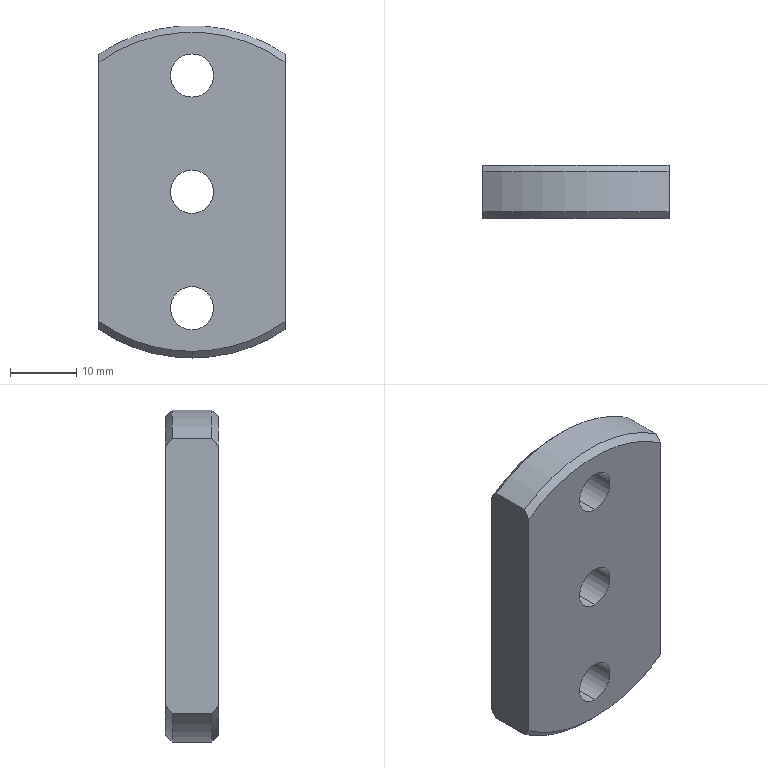Part | NX | features BREP 1 | 1 solid | 18 faces | box 28 x 8 x 50 mm | volume 9727 mm3 | cylinder 8 | cone 6 | plane 4 | commonest cylinder face diameters 6.5 x6 50 x2
STEP:
#1=CARTESIAN_POINT('',(-14.,0.,-19.494));
#2=VERTEX_POINT('',#1);
#3=CARTESIAN_POINT('',(0.,0.,-24.));
#4=VERTEX_POINT('',#3);
#5=CARTESIAN_POINT('',(0.,0.,0.));
#6=DIRECTION('',(0.,-1.,0.));
#7=DIRECTION('',(-0.5833,0.,-0.8122));
#8=AXIS2_PLACEMENT_3D('',#5,#6,#7);
#9=CIRCLE('',#8,24.);
#10=EDGE_CURVE('',#2,#4,#9,.T.);
#11=ORIENTED_EDGE('',*,*,#10,.T.);
#12=CARTESIAN_POINT('',(14.,0.,-19.494));
#13=VERTEX_POINT('',#12);
#14=CARTESIAN_POINT('',(0.,0.,0.));
#15=DIRECTION('',(0.,-1.,0.));
#16=DIRECTION('',(-0.5833,0.,-0.8122));
#17=AXIS2_PLACEMENT_3D('',#14,#15,#16);
#18=CIRCLE('',#17,24.);
#19=EDGE_CURVE('',#4,#13,#18,.T.);
#20=ORIENTED_EDGE('',*,*,#19,.T.);
#21=CARTESIAN_POINT('',(14.,0.,19.494));
#22=VERTEX_POINT('',#21);
#23=CARTESIAN_POINT('',(14.,0.,19.494));
#24=DIRECTION('',(0.,0.,-1.));
#25=VECTOR('',#24,1000.);
#26=LINE('',#23,#25);
#27=EDGE_CURVE('',#22,#13,#26,.T.);
#28=ORIENTED_EDGE('',*,*,#27,.F.);
#29=CARTESIAN_POINT('',(-14.,0.,19.494));
#30=VERTEX_POINT('',#29);
#31=CARTESIAN_POINT('',(0.,0.,0.));
#32=DIRECTION('',(0.,-1.,0.));
#33=DIRECTION('',(0.5833,0.,0.8122));
#34=AXIS2_PLACEMENT_3D('',#31,#32,#33);
#35=CIRCLE('',#34,24.);
#36=EDGE_CURVE('',#22,#30,#35,.T.);
#37=ORIENTED_EDGE('',*,*,#36,.T.);
#38=CARTESIAN_POINT('',(-14.,0.,19.494));
#39=DIRECTION('',(0.,0.,-1.));
#40=VECTOR('',#39,1000.);
#41=LINE('',#38,#40);
#42=EDGE_CURVE('',#30,#2,#41,.T.);
#43=ORIENTED_EDGE('',*,*,#42,.T.);
#44=EDGE_LOOP('',(#11,#20,#28,#37,#43));
#45=FACE_BOUND('',#44,.T.);
#46=CARTESIAN_POINT('',(0.,0.,-20.75));
#47=VERTEX_POINT('',#46);
#48=CARTESIAN_POINT('',(0.,0.,-14.25));
#49=VERTEX_POINT('',#48);
#50=CARTESIAN_POINT('',(0.,0.,-17.5));
#51=DIRECTION('',(0.,-1.,0.));
#52=DIRECTION('',(0.,0.,-1.));
#53=AXIS2_PLACEMENT_3D('',#50,#51,#52);
#54=CIRCLE('',#53,3.25);
#55=EDGE_CURVE('',#47,#49,#54,.T.);
#56=ORIENTED_EDGE('',*,*,#55,.F.);
#57=CARTESIAN_POINT('',(0.,0.,-17.5));
#58=DIRECTION('',(0.,-1.,0.));
#59=DIRECTION('',(0.,0.,1.));
#60=AXIS2_PLACEMENT_3D('',#57,#58,#59);
#61=CIRCLE('',#60,3.25);
#62=EDGE_CURVE('',#49,#47,#61,.T.);
#63=ORIENTED_EDGE('',*,*,#62,.F.);
#64=EDGE_LOOP('',(#56,#63));
#65=FACE_BOUND('',#64,.T.);
#66=CARTESIAN_POINT('',(0.,0.,20.75));
#67=VERTEX_POINT('',#66);
#68=CARTESIAN_POINT('',(0.,0.,14.25));
#69=VERTEX_POINT('',#68);
#70=CARTESIAN_POINT('',(0.,0.,17.5));
#71=DIRECTION('',(0.,-1.,0.));
#72=DIRECTION('',(0.,0.,1.));
#73=AXIS2_PLACEMENT_3D('',#70,#71,#72);
#74=CIRCLE('',#73,3.25);
#75=EDGE_CURVE('',#67,#69,#74,.T.);
#76=ORIENTED_EDGE('',*,*,#75,.F.);
#77=CARTESIAN_POINT('',(0.,0.,17.5));
#78=DIRECTION('',(0.,-1.,0.));
#79=DIRECTION('',(0.,0.,-1.));
#80=AXIS2_PLACEMENT_3D('',#77,#78,#79);
#81=CIRCLE('',#80,3.25);
#82=EDGE_CURVE('',#69,#67,#81,.T.);
#83=ORIENTED_EDGE('',*,*,#82,.F.);
#84=EDGE_LOOP('',(#76,#83));
#85=FACE_BOUND('',#84,.T.);
#86=CARTESIAN_POINT('',(0.,0.,3.25));
#87=VERTEX_POINT('',#86);
#88=CARTESIAN_POINT('',(0.,0.,-3.25));
#89=VERTEX_POINT('',#88);
#90=CARTESIAN_POINT('',(0.,0.,0.));
#91=DIRECTION('',(0.,-1.,0.));
#92=DIRECTION('',(0.,0.,1.));
#93=AXIS2_PLACEMENT_3D('',#90,#91,#92);
#94=CIRCLE('',#93,3.25);
#95=EDGE_CURVE('',#87,#89,#94,.T.);
#96=ORIENTED_EDGE('',*,*,#95,.F.);
#97=CARTESIAN_POINT('',(0.,0.,0.));
#98=DIRECTION('',(0.,-1.,0.));
#99=DIRECTION('',(0.,0.,-1.));
#100=AXIS2_PLACEMENT_3D('',#97,#98,#99);
#101=CIRCLE('',#100,3.25);
#102=EDGE_CURVE('',#89,#87,#101,.T.);
#103=ORIENTED_EDGE('',*,*,#102,.F.);
#104=EDGE_LOOP('',(#96,#103));
#105=FACE_BOUND('',#104,.T.);
#106=CARTESIAN_POINT('',(0.,0.,0.));
#107=DIRECTION('',(0.,1.,0.));
#108=DIRECTION('',(1.,0.,0.));
#109=AXIS2_PLACEMENT_3D('',#106,#107,#108);
#110=PLANE('',#109);
#111=ADVANCED_FACE('',(#45,#65,#85,#105),#110,.F.);
#112=CARTESIAN_POINT('',(0.,8.,3.25));
#113=VERTEX_POINT('',#112);
#114=CARTESIAN_POINT('',(0.,8.,3.25));
#115=DIRECTION('',(0.,-1.,0.));
#116=VECTOR('',#115,1000.);
#117=LINE('',#114,#116);
#118=EDGE_CURVE('',#87,#113,#117,.F.);
#119=ORIENTED_EDGE('',*,*,#118,.T.);
#120=CARTESIAN_POINT('',(0.,8.,-3.25));
#121=VERTEX_POINT('',#120);
#122=CARTESIAN_POINT('',(0.,8.,0.));
#123=DIRECTION('',(0.,-1.,0.));
#124=DIRECTION('',(0.,0.,-1.));
#125=AXIS2_PLACEMENT_3D('',#122,#123,#124);
#126=CIRCLE('',#125,3.25);
#127=EDGE_CURVE('',#121,#113,#126,.T.);
#128=ORIENTED_EDGE('',*,*,#127,.F.);
#129=CARTESIAN_POINT('',(0.,8.,-3.25));
#130=DIRECTION('',(0.,-1.,0.));
#131=VECTOR('',#130,1000.);
#132=LINE('',#129,#131);
#133=EDGE_CURVE('',#89,#121,#132,.F.);
#134=ORIENTED_EDGE('',*,*,#133,.F.);
#135=ORIENTED_EDGE('',*,*,#102,.T.);
#136=EDGE_LOOP('',(#119,#128,#134,#135));
#137=FACE_BOUND('',#136,.T.);
#138=CARTESIAN_POINT('',(0.,8.,0.));
#139=DIRECTION('',(0.,-1.,0.));
#140=DIRECTION('',(0.,0.,-1.));
#141=AXIS2_PLACEMENT_3D('',#138,#139,#140);
#142=CYLINDRICAL_SURFACE('',#141,3.25);
#143=ADVANCED_FACE('',(#137),#142,.F.);
#144=ORIENTED_EDGE('',*,*,#133,.T.);
#145=CARTESIAN_POINT('',(0.,8.,0.));
#146=DIRECTION('',(0.,-1.,0.));
#147=DIRECTION('',(0.,0.,1.));
#148=AXIS2_PLACEMENT_3D('',#145,#146,#147);
#149=CIRCLE('',#148,3.25);
#150=EDGE_CURVE('',#113,#121,#149,.T.);
#151=ORIENTED_EDGE('',*,*,#150,.F.);
#152=ORIENTED_EDGE('',*,*,#118,.F.);
#153=ORIENTED_EDGE('',*,*,#95,.T.);
#154=EDGE_LOOP('',(#144,#151,#152,#153));
#155=FACE_BOUND('',#154,.T.);
#156=CARTESIAN_POINT('',(0.,8.,0.));
#157=DIRECTION('',(0.,-1.,0.));
#158=DIRECTION('',(0.,0.,-1.));
#159=AXIS2_PLACEMENT_3D('',#156,#157,#158);
#160=CYLINDRICAL_SURFACE('',#159,3.25);
#161=ADVANCED_FACE('',(#155),#160,.F.);
#162=CARTESIAN_POINT('',(-14.,8.,19.494));
#163=VERTEX_POINT('',#162);
#164=CARTESIAN_POINT('',(14.,8.,19.494));
#165=VERTEX_POINT('',#164);
#166=CARTESIAN_POINT('',(0.,8.,0.));
#167=DIRECTION('',(0.,1.,0.));
#168=DIRECTION('',(-0.5833,0.,0.8122));
#169=AXIS2_PLACEMENT_3D('',#166,#167,#168);
#170=CIRCLE('',#169,24.);
#171=EDGE_CURVE('',#163,#165,#170,.T.);
#172=ORIENTED_EDGE('',*,*,#171,.T.);
#173=CARTESIAN_POINT('',(14.,8.,-19.494));
#174=VERTEX_POINT('',#173);
#175=CARTESIAN_POINT('',(14.,8.,19.494));
#176=DIRECTION('',(0.,0.,-1.));
#177=VECTOR('',#176,1000.);
#178=LINE('',#175,#177);
#179=EDGE_CURVE('',#165,#174,#178,.T.);
#180=ORIENTED_EDGE('',*,*,#179,.T.);
#181=CARTESIAN_POINT('',(0.,8.,-24.));
#182=VERTEX_POINT('',#181);
#183=CARTESIAN_POINT('',(0.,8.,0.));
#184=DIRECTION('',(0.,1.,0.));
#185=DIRECTION('',(0.5833,0.,-0.8122));
#186=AXIS2_PLACEMENT_3D('',#183,#184,#185);
#187=CIRCLE('',#186,24.);
#188=EDGE_CURVE('',#174,#182,#187,.T.);
#189=ORIENTED_EDGE('',*,*,#188,.T.);
#190=CARTESIAN_POINT('',(-14.,8.,-19.494));
#191=VERTEX_POINT('',#190);
#192=CARTESIAN_POINT('',(0.,8.,0.));
#193=DIRECTION('',(0.,1.,0.));
#194=DIRECTION('',(0.5833,0.,-0.8122));
#195=AXIS2_PLACEMENT_3D('',#192,#193,#194);
#196=CIRCLE('',#195,24.);
#197=EDGE_CURVE('',#182,#191,#196,.T.);
#198=ORIENTED_EDGE('',*,*,#197,.T.);
#199=CARTESIAN_POINT('',(-14.,8.,19.494));
#200=DIRECTION('',(0.,0.,-1.));
#201=VECTOR('',#200,1000.);
#202=LINE('',#199,#201);
#203=EDGE_CURVE('',#163,#191,#202,.T.);
#204=ORIENTED_EDGE('',*,*,#203,.F.);
#205=EDGE_LOOP('',(#172,#180,#189,#198,#204));
#206=FACE_BOUND('',#205,.T.);
#207=CARTESIAN_POINT('',(0.,8.,-20.75));
#208=VERTEX_POINT('',#207);
#209=CARTESIAN_POINT('',(0.,8.,-14.25));
#210=VERTEX_POINT('',#209);
#211=CARTESIAN_POINT('',(0.,8.,-17.5));
#212=DIRECTION('',(0.,-1.,0.));
#213=DIRECTION('',(0.,0.,-1.));
#214=AXIS2_PLACEMENT_3D('',#211,#212,#213);
#215=CIRCLE('',#214,3.25);
#216=EDGE_CURVE('',#208,#210,#215,.T.);
#217=ORIENTED_EDGE('',*,*,#216,.T.);
#218=CARTESIAN_POINT('',(0.,8.,-17.5));
#219=DIRECTION('',(0.,-1.,0.));
#220=DIRECTION('',(0.,0.,1.));
#221=AXIS2_PLACEMENT_3D('',#218,#219,#220);
#222=CIRCLE('',#221,3.25);
#223=EDGE_CURVE('',#210,#208,#222,.T.);
#224=ORIENTED_EDGE('',*,*,#223,.T.);
#225=EDGE_LOOP('',(#217,#224));
#226=FACE_BOUND('',#225,.T.);
#227=CARTESIAN_POINT('',(0.,8.,20.75));
#228=VERTEX_POINT('',#227);
#229=CARTESIAN_POINT('',(0.,8.,14.25));
#230=VERTEX_POINT('',#229);
#231=CARTESIAN_POINT('',(0.,8.,17.5));
#232=DIRECTION('',(0.,-1.,0.));
#233=DIRECTION('',(0.,0.,1.));
#234=AXIS2_PLACEMENT_3D('',#231,#232,#233);
#235=CIRCLE('',#234,3.25);
#236=EDGE_CURVE('',#228,#230,#235,.T.);
#237=ORIENTED_EDGE('',*,*,#236,.T.);
#238=CARTESIAN_POINT('',(0.,8.,17.5));
#239=DIRECTION('',(0.,-1.,0.));
#240=DIRECTION('',(0.,0.,-1.));
#241=AXIS2_PLACEMENT_3D('',#238,#239,#240);
#242=CIRCLE('',#241,3.25);
#243=EDGE_CURVE('',#230,#228,#242,.T.);
#244=ORIENTED_EDGE('',*,*,#243,.T.);
#245=EDGE_LOOP('',(#237,#244));
#246=FACE_BOUND('',#245,.T.);
#247=ORIENTED_EDGE('',*,*,#150,.T.);
#248=ORIENTED_EDGE('',*,*,#127,.T.);
#249=EDGE_LOOP('',(#247,#248));
#250=FACE_BOUND('',#249,.T.);
#251=CARTESIAN_POINT('',(0.,8.,0.));
#252=DIRECTION('',(0.,1.,0.));
#253=DIRECTION('',(1.,0.,0.));
#254=AXIS2_PLACEMENT_3D('',#251,#252,#253);
#255=PLANE('',#254);
#256=ADVANCED_FACE('',(#206,#226,#246,#250),#255,.T.);
#257=CARTESIAN_POINT('',(0.,8.,-20.75));
#258=DIRECTION('',(0.,-1.,0.));
#259=VECTOR('',#258,1000.);
#260=LINE('',#257,#259);
#261=EDGE_CURVE('',#208,#47,#260,.T.);
#262=ORIENTED_EDGE('',*,*,#261,.F.);
#263=ORIENTED_EDGE('',*,*,#223,.F.);
#264=CARTESIAN_POINT('',(0.,8.,-14.25));
#265=DIRECTION('',(0.,-1.,0.));
#266=VECTOR('',#265,1000.);
#267=LINE('',#264,#266);
#268=EDGE_CURVE('',#210,#49,#267,.T.);
#269=ORIENTED_EDGE('',*,*,#268,.T.);
#270=ORIENTED_EDGE('',*,*,#62,.T.);
#271=EDGE_LOOP('',(#262,#263,#269,#270));
#272=FACE_BOUND('',#271,.T.);
#273=CARTESIAN_POINT('',(0.,8.,-17.5));
#274=DIRECTION('',(0.,-1.,0.));
#275=DIRECTION('',(0.,0.,1.));
#276=AXIS2_PLACEMENT_3D('',#273,#274,#275);
#277=CYLINDRICAL_SURFACE('',#276,3.25);
#278=ADVANCED_FACE('',(#272),#277,.F.);
#279=ORIENTED_EDGE('',*,*,#268,.F.);
#280=ORIENTED_EDGE('',*,*,#216,.F.);
#281=ORIENTED_EDGE('',*,*,#261,.T.);
#282=ORIENTED_EDGE('',*,*,#55,.T.);
#283=EDGE_LOOP('',(#279,#280,#281,#282));
#284=FACE_BOUND('',#283,.T.);
#285=CARTESIAN_POINT('',(0.,8.,-17.5));
#286=DIRECTION('',(0.,-1.,0.));
#287=DIRECTION('',(0.,0.,1.));
#288=AXIS2_PLACEMENT_3D('',#285,#286,#287);
#289=CYLINDRICAL_SURFACE('',#288,3.25);
#290=ADVANCED_FACE('',(#284),#289,.F.);
#291=CARTESIAN_POINT('',(0.,8.,20.75));
#292=DIRECTION('',(0.,-1.,0.));
#293=VECTOR('',#292,1000.);
#294=LINE('',#291,#293);
#295=EDGE_CURVE('',#67,#228,#294,.F.);
#296=ORIENTED_EDGE('',*,*,#295,.T.);
#297=ORIENTED_EDGE('',*,*,#243,.F.);
#298=CARTESIAN_POINT('',(0.,8.,14.25));
#299=DIRECTION('',(0.,-1.,0.));
#300=VECTOR('',#299,1000.);
#301=LINE('',#298,#300);
#302=EDGE_CURVE('',#69,#230,#301,.F.);
#303=ORIENTED_EDGE('',*,*,#302,.F.);
#304=ORIENTED_EDGE('',*,*,#82,.T.);
#305=EDGE_LOOP('',(#296,#297,#303,#304));
#306=FACE_BOUND('',#305,.T.);
#307=CARTESIAN_POINT('',(0.,8.,17.5));
#308=DIRECTION('',(0.,-1.,0.));
#309=DIRECTION('',(0.,0.,-1.));
#310=AXIS2_PLACEMENT_3D('',#307,#308,#309);
#311=CYLINDRICAL_SURFACE('',#310,3.25);
#312=ADVANCED_FACE('',(#306),#311,.F.);
#313=ORIENTED_EDGE('',*,*,#302,.T.);
#314=ORIENTED_EDGE('',*,*,#236,.F.);
#315=ORIENTED_EDGE('',*,*,#295,.F.);
#316=ORIENTED_EDGE('',*,*,#75,.T.);
#317=EDGE_LOOP('',(#313,#314,#315,#316));
#318=FACE_BOUND('',#317,.T.);
#319=CARTESIAN_POINT('',(0.,8.,17.5));
#320=DIRECTION('',(0.,-1.,0.));
#321=DIRECTION('',(0.,0.,-1.));
#322=AXIS2_PLACEMENT_3D('',#319,#320,#321);
#323=CYLINDRICAL_SURFACE('',#322,3.25);
#324=ADVANCED_FACE('',(#318),#323,.F.);
#325=CARTESIAN_POINT('',(-14.,1.,20.712));
#326=VERTEX_POINT('',#325);
#327=CARTESIAN_POINT('',(-14.,0.,19.494));
#328=CARTESIAN_POINT('',(-14.,0.1077,19.626));
#329=CARTESIAN_POINT('',(-14.,0.3254,19.893));
#330=CARTESIAN_POINT('',(-14.,0.6586,20.299));
#331=CARTESIAN_POINT('',(-14.,0.8854,20.574));
#332=CARTESIAN_POINT('',(-14.,1.,20.712));
#333=B_SPLINE_CURVE_WITH_KNOTS('',3,(#327,#328,#329,#330,#331,#332),.UNSPECIFIED.,.F.,.F.,(4,1,1,4),(0.,0.3333,0.6667,1.),.UNSPECIFIED.);
#334=EDGE_CURVE('',#30,#326,#333,.T.);
#335=ORIENTED_EDGE('',*,*,#334,.T.);
#336=CARTESIAN_POINT('',(-14.,7.,20.712));
#337=VERTEX_POINT('',#336);
#338=CARTESIAN_POINT('',(-14.,1.,20.712));
#339=DIRECTION('',(0.,1.,0.));
#340=VECTOR('',#339,1000.);
#341=LINE('',#338,#340);
#342=EDGE_CURVE('',#326,#337,#341,.T.);
#343=ORIENTED_EDGE('',*,*,#342,.T.);
#344=CARTESIAN_POINT('',(-14.,7.,20.712));
#345=CARTESIAN_POINT('',(-14.,7.115,20.574));
#346=CARTESIAN_POINT('',(-14.,7.341,20.299));
#347=CARTESIAN_POINT('',(-14.,7.675,19.893));
#348=CARTESIAN_POINT('',(-14.,7.892,19.626));
#349=CARTESIAN_POINT('',(-14.,8.,19.494));
#350=B_SPLINE_CURVE_WITH_KNOTS('',3,(#344,#345,#346,#347,#348,#349),.UNSPECIFIED.,.F.,.F.,(4,1,1,4),(0.,0.3333,0.6667,1.),.UNSPECIFIED.);
#351=EDGE_CURVE('',#337,#163,#350,.T.);
#352=ORIENTED_EDGE('',*,*,#351,.T.);
#353=ORIENTED_EDGE('',*,*,#203,.T.);
#354=CARTESIAN_POINT('',(-14.,7.,-20.712));
#355=VERTEX_POINT('',#354);
#356=CARTESIAN_POINT('',(-14.,8.,-19.494));
#357=CARTESIAN_POINT('',(-14.,7.892,-19.626));
#358=CARTESIAN_POINT('',(-14.,7.675,-19.893));
#359=CARTESIAN_POINT('',(-14.,7.341,-20.299));
#360=CARTESIAN_POINT('',(-14.,7.115,-20.574));
#361=CARTESIAN_POINT('',(-14.,7.,-20.712));
#362=B_SPLINE_CURVE_WITH_KNOTS('',3,(#356,#357,#358,#359,#360,#361),.UNSPECIFIED.,.F.,.F.,(4,1,1,4),(0.,0.3333,0.6667,1.),.UNSPECIFIED.);
#363=EDGE_CURVE('',#191,#355,#362,.T.);
#364=ORIENTED_EDGE('',*,*,#363,.T.);
#365=CARTESIAN_POINT('',(-14.,1.,-20.712));
#366=VERTEX_POINT('',#365);
#367=CARTESIAN_POINT('',(-14.,1.,-20.712));
#368=DIRECTION('',(0.,1.,0.));
#369=VECTOR('',#368,1000.);
#370=LINE('',#367,#369);
#371=EDGE_CURVE('',#366,#355,#370,.T.);
#372=ORIENTED_EDGE('',*,*,#371,.F.);
#373=CARTESIAN_POINT('',(-14.,1.,-20.712));
#374=CARTESIAN_POINT('',(-14.,0.8855,-20.574));
#375=CARTESIAN_POINT('',(-14.,0.6587,-20.299));
#376=CARTESIAN_POINT('',(-14.,0.3254,-19.893));
#377=CARTESIAN_POINT('',(-14.,0.1077,-19.626));
#378=CARTESIAN_POINT('',(-14.,0.,-19.494));
#379=B_SPLINE_CURVE_WITH_KNOTS('',3,(#373,#374,#375,#376,#377,#378),.UNSPECIFIED.,.F.,.F.,(4,1,1,4),(0.,0.3333,0.6667,1.),.UNSPECIFIED.);
#380=EDGE_CURVE('',#366,#2,#379,.T.);
#381=ORIENTED_EDGE('',*,*,#380,.T.);
#382=ORIENTED_EDGE('',*,*,#42,.F.);
#383=EDGE_LOOP('',(#335,#343,#352,#353,#364,#372,#381,#382));
#384=FACE_BOUND('',#383,.T.);
#385=CARTESIAN_POINT('',(-14.,8.,25.));
#386=DIRECTION('',(1.,0.,0.));
#387=DIRECTION('',(0.,1.,0.));
#388=AXIS2_PLACEMENT_3D('',#385,#386,#387);
#389=PLANE('',#388);
#390=ADVANCED_FACE('',(#384),#389,.F.);
#391=CARTESIAN_POINT('',(0.,1.,-25.));
#392=VERTEX_POINT('',#391);
#393=CARTESIAN_POINT('',(0.,0.5,-24.5));
#394=DIRECTION('',(0.,0.7071,-0.7071));
#395=VECTOR('',#394,1000.);
#396=LINE('',#393,#395);
#397=EDGE_CURVE('',#4,#392,#396,.T.);
#398=ORIENTED_EDGE('',*,*,#397,.F.);
#399=ORIENTED_EDGE('',*,*,#10,.F.);
#400=ORIENTED_EDGE('',*,*,#380,.F.);
#401=CARTESIAN_POINT('',(0.,1.,0.));
#402=DIRECTION('',(0.,-1.,0.));
#403=DIRECTION('',(-0.56,0.,-0.8285));
#404=AXIS2_PLACEMENT_3D('',#401,#402,#403);
#405=CIRCLE('',#404,25.);
#406=EDGE_CURVE('',#366,#392,#405,.T.);
#407=ORIENTED_EDGE('',*,*,#406,.T.);
#408=EDGE_LOOP('',(#398,#399,#400,#407));
#409=FACE_BOUND('',#408,.T.);
#410=CARTESIAN_POINT('',(0.,0.5,0.));
#411=DIRECTION('',(0.,1.,0.));
#412=DIRECTION('',(0.,0.,-1.));
#413=AXIS2_PLACEMENT_3D('',#410,#411,#412);
#414=CONICAL_SURFACE('',#413,24.5,0.7854);
#415=ADVANCED_FACE('',(#409),#414,.T.);
#416=CARTESIAN_POINT('',(14.,1.,-20.712));
#417=VERTEX_POINT('',#416);
#418=CARTESIAN_POINT('',(14.,0.,-19.494));
#419=CARTESIAN_POINT('',(14.,0.1077,-19.626));
#420=CARTESIAN_POINT('',(14.,0.3254,-19.893));
#421=CARTESIAN_POINT('',(14.,0.6586,-20.299));
#422=CARTESIAN_POINT('',(14.,0.8854,-20.574));
#423=CARTESIAN_POINT('',(14.,1.,-20.712));
#424=B_SPLINE_CURVE_WITH_KNOTS('',3,(#418,#419,#420,#421,#422,#423),.UNSPECIFIED.,.F.,.F.,(4,1,1,4),(0.,0.3333,0.6667,1.),.UNSPECIFIED.);
#425=EDGE_CURVE('',#13,#417,#424,.T.);
#426=ORIENTED_EDGE('',*,*,#425,.T.);
#427=CARTESIAN_POINT('',(14.,7.,-20.712));
#428=VERTEX_POINT('',#427);
#429=CARTESIAN_POINT('',(14.,1.,-20.712));
#430=DIRECTION('',(0.,1.,0.));
#431=VECTOR('',#430,1000.);
#432=LINE('',#429,#431);
#433=EDGE_CURVE('',#417,#428,#432,.T.);
#434=ORIENTED_EDGE('',*,*,#433,.T.);
#435=CARTESIAN_POINT('',(14.,7.,-20.712));
#436=CARTESIAN_POINT('',(14.,7.115,-20.574));
#437=CARTESIAN_POINT('',(14.,7.341,-20.299));
#438=CARTESIAN_POINT('',(14.,7.675,-19.893));
#439=CARTESIAN_POINT('',(14.,7.892,-19.626));
#440=CARTESIAN_POINT('',(14.,8.,-19.494));
#441=B_SPLINE_CURVE_WITH_KNOTS('',3,(#435,#436,#437,#438,#439,#440),.UNSPECIFIED.,.F.,.F.,(4,1,1,4),(0.,0.3333,0.6667,1.),.UNSPECIFIED.);
#442=EDGE_CURVE('',#428,#174,#441,.T.);
#443=ORIENTED_EDGE('',*,*,#442,.T.);
#444=ORIENTED_EDGE('',*,*,#179,.F.);
#445=CARTESIAN_POINT('',(14.,7.,20.712));
#446=VERTEX_POINT('',#445);
#447=CARTESIAN_POINT('',(14.,8.,19.494));
#448=CARTESIAN_POINT('',(14.,7.892,19.626));
#449=CARTESIAN_POINT('',(14.,7.675,19.893));
#450=CARTESIAN_POINT('',(14.,7.341,20.299));
#451=CARTESIAN_POINT('',(14.,7.115,20.574));
#452=CARTESIAN_POINT('',(14.,7.,20.712));
#453=B_SPLINE_CURVE_WITH_KNOTS('',3,(#447,#448,#449,#450,#451,#452),.UNSPECIFIED.,.F.,.F.,(4,1,1,4),(0.,0.3333,0.6667,1.),.UNSPECIFIED.);
#454=EDGE_CURVE('',#165,#446,#453,.T.);
#455=ORIENTED_EDGE('',*,*,#454,.T.);
#456=CARTESIAN_POINT('',(14.,1.,20.712));
#457=VERTEX_POINT('',#456);
#458=CARTESIAN_POINT('',(14.,1.,20.712));
#459=DIRECTION('',(0.,1.,0.));
#460=VECTOR('',#459,1000.);
#461=LINE('',#458,#460);
#462=EDGE_CURVE('',#457,#446,#461,.T.);
#463=ORIENTED_EDGE('',*,*,#462,.F.);
#464=CARTESIAN_POINT('',(14.,1.,20.712));
#465=CARTESIAN_POINT('',(14.,0.8855,20.574));
#466=CARTESIAN_POINT('',(14.,0.6587,20.299));
#467=CARTESIAN_POINT('',(14.,0.3254,19.893));
#468=CARTESIAN_POINT('',(14.,0.1077,19.626));
#469=CARTESIAN_POINT('',(14.,0.,19.494));
#470=B_SPLINE_CURVE_WITH_KNOTS('',3,(#464,#465,#466,#467,#468,#469),.UNSPECIFIED.,.F.,.F.,(4,1,1,4),(0.,0.3333,0.6667,1.),.UNSPECIFIED.);
#471=EDGE_CURVE('',#457,#22,#470,.T.);
#472=ORIENTED_EDGE('',*,*,#471,.T.);
#473=ORIENTED_EDGE('',*,*,#27,.T.);
#474=EDGE_LOOP('',(#426,#434,#443,#444,#455,#463,#472,#473));
#475=FACE_BOUND('',#474,.T.);
#476=CARTESIAN_POINT('',(14.,8.,-25.));
#477=DIRECTION('',(-1.,0.,0.));
#478=DIRECTION('',(0.,0.,1.));
#479=AXIS2_PLACEMENT_3D('',#476,#477,#478);
#480=PLANE('',#479);
#481=ADVANCED_FACE('',(#475),#480,.F.);
#482=ORIENTED_EDGE('',*,*,#36,.F.);
#483=ORIENTED_EDGE('',*,*,#471,.F.);
#484=CARTESIAN_POINT('',(0.,1.,0.));
#485=DIRECTION('',(0.,-1.,0.));
#486=DIRECTION('',(0.56,0.,0.8285));
#487=AXIS2_PLACEMENT_3D('',#484,#485,#486);
#488=CIRCLE('',#487,25.);
#489=EDGE_CURVE('',#457,#326,#488,.T.);
#490=ORIENTED_EDGE('',*,*,#489,.T.);
#491=ORIENTED_EDGE('',*,*,#334,.F.);
#492=EDGE_LOOP('',(#482,#483,#490,#491));
#493=FACE_BOUND('',#492,.T.);
#494=CARTESIAN_POINT('',(0.,0.5,0.));
#495=DIRECTION('',(0.,1.,0.));
#496=DIRECTION('',(0.,0.,-1.));
#497=AXIS2_PLACEMENT_3D('',#494,#495,#496);
#498=CONICAL_SURFACE('',#497,24.5,0.7854);
#499=ADVANCED_FACE('',(#493),#498,.T.);
#500=ORIENTED_EDGE('',*,*,#489,.F.);
#501=ORIENTED_EDGE('',*,*,#462,.T.);
#502=CARTESIAN_POINT('',(0.,7.,0.));
#503=DIRECTION('',(0.,1.,0.));
#504=DIRECTION('',(-0.56,0.,0.8285));
#505=AXIS2_PLACEMENT_3D('',#502,#503,#504);
#506=CIRCLE('',#505,25.);
#507=EDGE_CURVE('',#337,#446,#506,.T.);
#508=ORIENTED_EDGE('',*,*,#507,.F.);
#509=ORIENTED_EDGE('',*,*,#342,.F.);
#510=EDGE_LOOP('',(#500,#501,#508,#509));
#511=FACE_BOUND('',#510,.T.);
#512=CARTESIAN_POINT('',(0.,0.,0.));
#513=DIRECTION('',(0.,1.,0.));
#514=DIRECTION('',(1.,0.,0.));
#515=AXIS2_PLACEMENT_3D('',#512,#513,#514);
#516=CYLINDRICAL_SURFACE('',#515,25.);
#517=ADVANCED_FACE('',(#511),#516,.T.);
#518=ORIENTED_EDGE('',*,*,#507,.T.);
#519=ORIENTED_EDGE('',*,*,#454,.F.);
#520=ORIENTED_EDGE('',*,*,#171,.F.);
#521=ORIENTED_EDGE('',*,*,#351,.F.);
#522=EDGE_LOOP('',(#518,#519,#520,#521));
#523=FACE_BOUND('',#522,.T.);
#524=CARTESIAN_POINT('',(0.,7.5,0.));
#525=DIRECTION('',(0.,-1.,0.));
#526=DIRECTION('',(0.,0.,-1.));
#527=AXIS2_PLACEMENT_3D('',#524,#525,#526);
#528=CONICAL_SURFACE('',#527,24.5,0.7854);
#529=ADVANCED_FACE('',(#523),#528,.T.);
#530=CARTESIAN_POINT('',(0.,7.,-25.));
#531=VERTEX_POINT('',#530);
#532=CARTESIAN_POINT('',(0.,7.5,-24.5));
#533=DIRECTION('',(0.,-0.7071,-0.7071));
#534=VECTOR('',#533,1000.);
#535=LINE('',#532,#534);
#536=EDGE_CURVE('',#182,#531,#535,.T.);
#537=ORIENTED_EDGE('',*,*,#536,.F.);
#538=ORIENTED_EDGE('',*,*,#188,.F.);
#539=ORIENTED_EDGE('',*,*,#442,.F.);
#540=CARTESIAN_POINT('',(0.,7.,0.));
#541=DIRECTION('',(0.,1.,0.));
#542=DIRECTION('',(0.56,0.,-0.8285));
#543=AXIS2_PLACEMENT_3D('',#540,#541,#542);
#544=CIRCLE('',#543,25.);
#545=EDGE_CURVE('',#428,#531,#544,.T.);
#546=ORIENTED_EDGE('',*,*,#545,.T.);
#547=EDGE_LOOP('',(#537,#538,#539,#546));
#548=FACE_BOUND('',#547,.T.);
#549=CARTESIAN_POINT('',(0.,7.5,0.));
#550=DIRECTION('',(0.,-1.,0.));
#551=DIRECTION('',(0.,0.,-1.));
#552=AXIS2_PLACEMENT_3D('',#549,#550,#551);
#553=CONICAL_SURFACE('',#552,24.5,0.7854);
#554=ADVANCED_FACE('',(#548),#553,.T.);
#555=ORIENTED_EDGE('',*,*,#545,.F.);
#556=ORIENTED_EDGE('',*,*,#433,.F.);
#557=CARTESIAN_POINT('',(0.,1.,0.));
#558=DIRECTION('',(0.,-1.,0.));
#559=DIRECTION('',(-0.56,0.,-0.8285));
#560=AXIS2_PLACEMENT_3D('',#557,#558,#559);
#561=CIRCLE('',#560,25.);
#562=EDGE_CURVE('',#392,#417,#561,.T.);
#563=ORIENTED_EDGE('',*,*,#562,.F.);
#564=ORIENTED_EDGE('',*,*,#406,.F.);
#565=ORIENTED_EDGE('',*,*,#371,.T.);
#566=CARTESIAN_POINT('',(0.,7.,0.));
#567=DIRECTION('',(0.,1.,0.));
#568=DIRECTION('',(0.56,0.,-0.8285));
#569=AXIS2_PLACEMENT_3D('',#566,#567,#568);
#570=CIRCLE('',#569,25.);
#571=EDGE_CURVE('',#531,#355,#570,.T.);
#572=ORIENTED_EDGE('',*,*,#571,.F.);
#573=EDGE_LOOP('',(#555,#556,#563,#564,#565,#572));
#574=FACE_BOUND('',#573,.T.);
#575=CARTESIAN_POINT('',(0.,0.,0.));
#576=DIRECTION('',(0.,1.,0.));
#577=DIRECTION('',(1.,0.,0.));
#578=AXIS2_PLACEMENT_3D('',#575,#576,#577);
#579=CYLINDRICAL_SURFACE('',#578,25.);
#580=ADVANCED_FACE('',(#574),#579,.T.);
#581=ORIENTED_EDGE('',*,*,#197,.F.);
#582=ORIENTED_EDGE('',*,*,#536,.T.);
#583=ORIENTED_EDGE('',*,*,#571,.T.);
#584=ORIENTED_EDGE('',*,*,#363,.F.);
#585=EDGE_LOOP('',(#581,#582,#583,#584));
#586=FACE_BOUND('',#585,.T.);
#587=CARTESIAN_POINT('',(0.,7.5,0.));
#588=DIRECTION('',(0.,-1.,0.));
#589=DIRECTION('',(0.,0.,-1.));
#590=AXIS2_PLACEMENT_3D('',#587,#588,#589);
#591=CONICAL_SURFACE('',#590,24.5,0.7854);
#592=ADVANCED_FACE('',(#586),#591,.T.);
#593=ORIENTED_EDGE('',*,*,#19,.F.);
#594=ORIENTED_EDGE('',*,*,#397,.T.);
#595=ORIENTED_EDGE('',*,*,#562,.T.);
#596=ORIENTED_EDGE('',*,*,#425,.F.);
#597=EDGE_LOOP('',(#593,#594,#595,#596));
#598=FACE_BOUND('',#597,.T.);
#599=CARTESIAN_POINT('',(0.,0.5,0.));
#600=DIRECTION('',(0.,1.,0.));
#601=DIRECTION('',(0.,0.,-1.));
#602=AXIS2_PLACEMENT_3D('',#599,#600,#601);
#603=CONICAL_SURFACE('',#602,24.5,0.7854);
#604=ADVANCED_FACE('',(#598),#603,.T.);
#605=CLOSED_SHELL('',(#111,#143,#161,#256,#278,#290,#312,#324,#390,#415,#481,#499,#517,#529,#554,#580,#592,#604));
#606=MANIFOLD_SOLID_BREP('',#605);
#607=(LENGTH_UNIT()NAMED_UNIT(*)SI_UNIT(.MILLI.,.METRE.));
#608=UNCERTAINTY_MEASURE_WITH_UNIT(LENGTH_MEASURE(0.00001),#607,'','');
#609=(NAMED_UNIT(*)PLANE_ANGLE_UNIT()SI_UNIT($,.RADIAN.));
#610=(NAMED_UNIT(*)SI_UNIT($,.STERADIAN.)SOLID_ANGLE_UNIT());
#611=(GEOMETRIC_REPRESENTATION_CONTEXT(3)GLOBAL_UNCERTAINTY_ASSIGNED_CONTEXT((#608))GLOBAL_UNIT_ASSIGNED_CONTEXT((#607,#609,#610))REPRESENTATION_CONTEXT('',''));
#612=ADVANCED_BREP_SHAPE_REPRESENTATION('',(#606),#611);